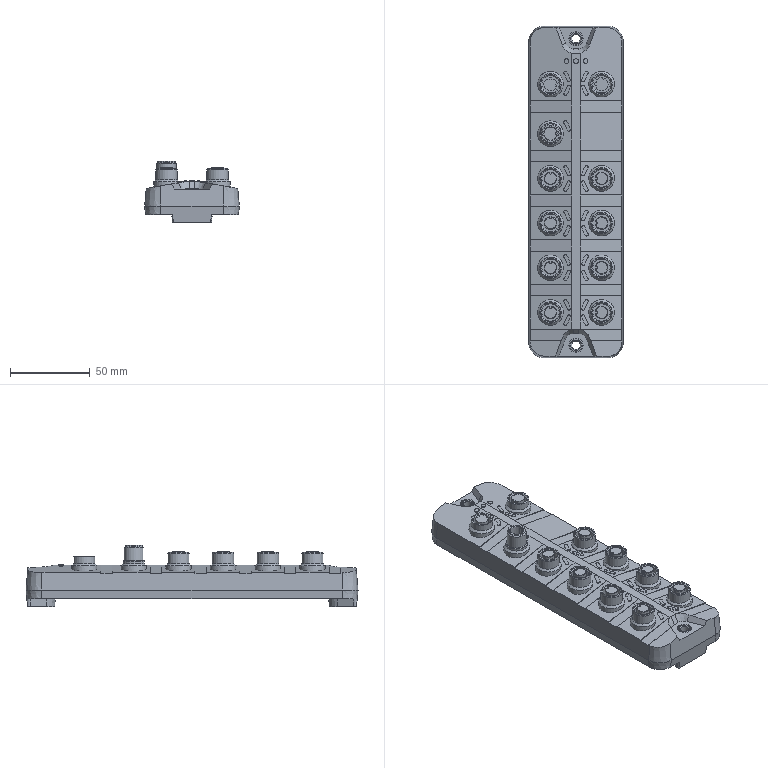Part | NX | features BREP 1 | 1 solid | 412 faces | box 59.3 x 208 x 38.25 mm | volume 240044 mm3 | plane 183 | cylinder 165 | cone 56 | torus 8 | commonest cylinder face diameters 2 x42 21.4 x21 25.4 x21 1.2 x17 13.5 x11 16 x11